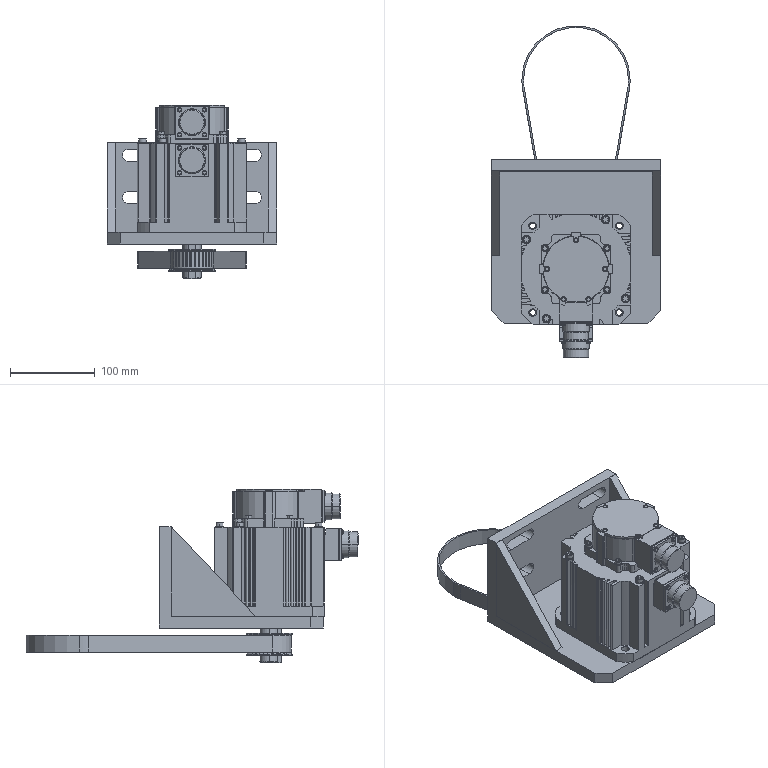Part | SolidWorks | 6 solids | 1057 faces | box 200 x 393 x 205 mm | volume 2855185 mm3 | cylinder 519 | plane 440 | cone 52 | spline 46 | commonest cylinder face diameters 1 x90 0.5 x85 3.155 x48 49.79 x33 2 x30 4 x24